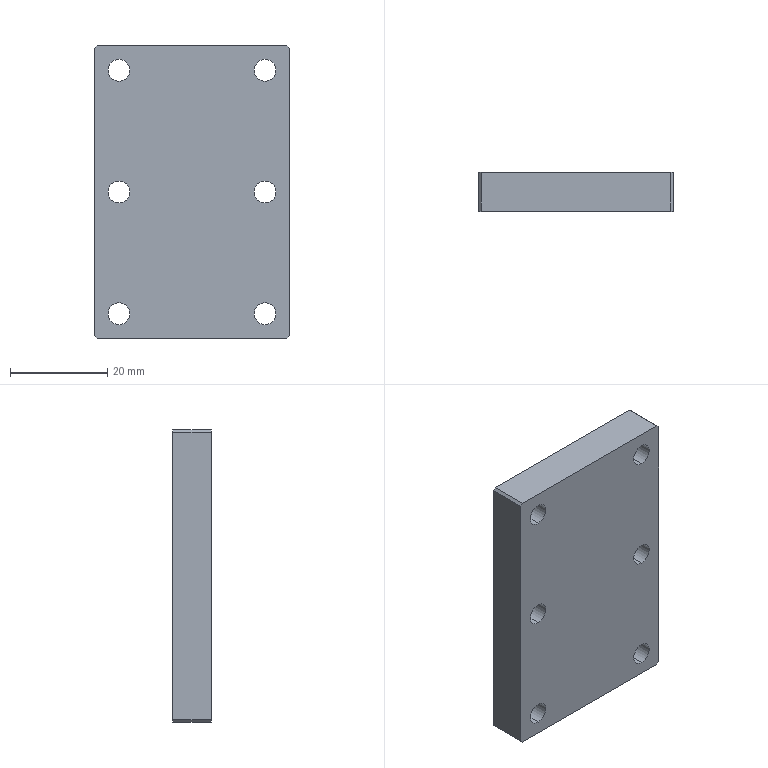Part | STEP file | PN_0017 Mount electronic clip blade pressure plate 2 | 1 solid | 22 faces | box 40 x 8 x 60 mm | volume 18433 mm3 | cylinder 12 | plane 10 | commonest cylinder face diameters 4.5 x12